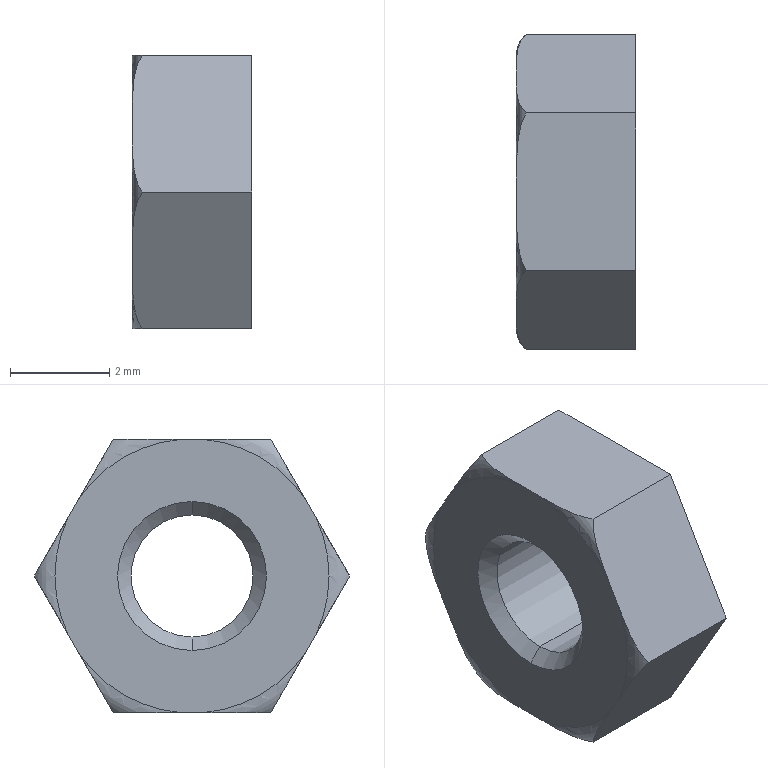Part | SolidWorks | features RefAxis 3, 3DProfileFeature 1, ICE 1, RevCut 1, Revolution 1 | 1 solid | 20 faces | box 2.4 x 6.351 x 5.5 mm | volume 50.814 mm3 | plane 8 | torus 6 | cone 4 | cylinder 2 | commonest cylinder face diameters 2.459 x2
STEP:
#1=CARTESIAN_POINT('',(0.9295,0.,-1.23));
#2=VERTEX_POINT('',#1);
#3=CARTESIAN_POINT('',(0.9295,0.,1.23));
#4=VERTEX_POINT('',#3);
#5=CARTESIAN_POINT('',(0.9295,0.,0.));
#6=DIRECTION('',(-1.,0.,0.));
#7=DIRECTION('',(0.,0.,1.));
#8=AXIS2_PLACEMENT_3D('',#5,#6,#7);
#9=CIRCLE('',#8,1.23);
#10=EDGE_CURVE('',#2,#4,#9,.T.);
#11=ORIENTED_EDGE('',*,*,#10,.T.);
#12=CARTESIAN_POINT('',(1.2,0.,1.5));
#13=VERTEX_POINT('',#12);
#14=CARTESIAN_POINT('',(1.2,0.,1.5));
#15=DIRECTION('',(0.7071,0.,0.7071));
#16=VECTOR('',#15,1000.);
#17=LINE('',#14,#16);
#18=EDGE_CURVE('',#4,#13,#17,.T.);
#19=ORIENTED_EDGE('',*,*,#18,.T.);
#20=CARTESIAN_POINT('',(1.2,0.,-1.5));
#21=VERTEX_POINT('',#20);
#22=CARTESIAN_POINT('',(1.2,0.,0.));
#23=DIRECTION('',(-1.,0.,0.));
#24=DIRECTION('',(0.,0.,1.));
#25=AXIS2_PLACEMENT_3D('',#22,#23,#24);
#26=CIRCLE('',#25,1.5);
#27=EDGE_CURVE('',#21,#13,#26,.T.);
#28=ORIENTED_EDGE('',*,*,#27,.F.);
#29=CARTESIAN_POINT('',(1.2,0.,-1.5));
#30=DIRECTION('',(0.7071,0.,-0.7071));
#31=VECTOR('',#30,1000.);
#32=LINE('',#29,#31);
#33=EDGE_CURVE('',#2,#21,#32,.T.);
#34=ORIENTED_EDGE('',*,*,#33,.F.);
#35=EDGE_LOOP('',(#11,#19,#28,#34));
#36=FACE_OUTER_BOUND('',#35,.T.);
#37=CARTESIAN_POINT('',(1.2,0.,0.));
#38=DIRECTION('',(1.,0.,0.));
#39=DIRECTION('',(0.,0.,-1.));
#40=AXIS2_PLACEMENT_3D('',#37,#38,#39);
#41=CONICAL_SURFACE('',#40,1.5,0.7854);
#42=ADVANCED_FACE('',(#36),#41,.F.);
#43=ORIENTED_EDGE('',*,*,#10,.F.);
#44=CARTESIAN_POINT('',(-0.9295,0.,-1.23));
#45=VERTEX_POINT('',#44);
#46=CARTESIAN_POINT('',(1.2,0.,-1.23));
#47=DIRECTION('',(-1.,0.,0.));
#48=VECTOR('',#47,1000.);
#49=LINE('',#46,#48);
#50=EDGE_CURVE('',#2,#45,#49,.T.);
#51=ORIENTED_EDGE('',*,*,#50,.T.);
#52=CARTESIAN_POINT('',(-0.9295,0.,1.23));
#53=VERTEX_POINT('',#52);
#54=CARTESIAN_POINT('',(-0.9295,0.,0.));
#55=DIRECTION('',(-1.,0.,0.));
#56=DIRECTION('',(0.,0.,1.));
#57=AXIS2_PLACEMENT_3D('',#54,#55,#56);
#58=CIRCLE('',#57,1.23);
#59=EDGE_CURVE('',#45,#53,#58,.T.);
#60=ORIENTED_EDGE('',*,*,#59,.T.);
#61=CARTESIAN_POINT('',(1.2,0.,1.23));
#62=DIRECTION('',(-1.,0.,0.));
#63=VECTOR('',#62,1000.);
#64=LINE('',#61,#63);
#65=EDGE_CURVE('',#4,#53,#64,.T.);
#66=ORIENTED_EDGE('',*,*,#65,.F.);
#67=EDGE_LOOP('',(#43,#51,#60,#66));
#68=FACE_OUTER_BOUND('',#67,.T.);
#69=CARTESIAN_POINT('',(1.2,0.,0.));
#70=DIRECTION('',(-1.,0.,0.));
#71=DIRECTION('',(0.,0.,1.));
#72=AXIS2_PLACEMENT_3D('',#69,#70,#71);
#73=CYLINDRICAL_SURFACE('',#72,1.23);
#74=ADVANCED_FACE('',(#68),#73,.F.);
#75=ORIENTED_EDGE('',*,*,#59,.F.);
#76=CARTESIAN_POINT('',(-1.2,0.,-1.5));
#77=VERTEX_POINT('',#76);
#78=CARTESIAN_POINT('',(-0.9295,0.,-1.23));
#79=DIRECTION('',(-0.7071,0.,-0.7071));
#80=VECTOR('',#79,1000.);
#81=LINE('',#78,#80);
#82=EDGE_CURVE('',#45,#77,#81,.T.);
#83=ORIENTED_EDGE('',*,*,#82,.T.);
#84=CARTESIAN_POINT('',(-1.2,0.,1.5));
#85=VERTEX_POINT('',#84);
#86=CARTESIAN_POINT('',(-1.2,0.,0.));
#87=DIRECTION('',(-1.,0.,0.));
#88=DIRECTION('',(0.,0.,1.));
#89=AXIS2_PLACEMENT_3D('',#86,#87,#88);
#90=CIRCLE('',#89,1.5);
#91=EDGE_CURVE('',#77,#85,#90,.T.);
#92=ORIENTED_EDGE('',*,*,#91,.T.);
#93=CARTESIAN_POINT('',(-0.9295,0.,1.23));
#94=DIRECTION('',(-0.7071,0.,0.7071));
#95=VECTOR('',#94,1000.);
#96=LINE('',#93,#95);
#97=EDGE_CURVE('',#53,#85,#96,.T.);
#98=ORIENTED_EDGE('',*,*,#97,.F.);
#99=EDGE_LOOP('',(#75,#83,#92,#98));
#100=FACE_OUTER_BOUND('',#99,.T.);
#101=CARTESIAN_POINT('',(-0.9295,0.,0.));
#102=DIRECTION('',(-1.,0.,0.));
#103=DIRECTION('',(0.,0.,1.));
#104=AXIS2_PLACEMENT_3D('',#101,#102,#103);
#105=CONICAL_SURFACE('',#104,1.23,0.7854);
#106=ADVANCED_FACE('',(#100),#105,.F.);
#107=CARTESIAN_POINT('',(-1.2,0.,0.));
#108=DIRECTION('',(-1.,0.,0.));
#109=DIRECTION('',(0.,0.,1.));
#110=AXIS2_PLACEMENT_3D('',#107,#108,#109);
#111=CIRCLE('',#110,1.5);
#112=EDGE_CURVE('',#85,#77,#111,.T.);
#113=ORIENTED_EDGE('',*,*,#112,.F.);
#114=ORIENTED_EDGE('',*,*,#91,.F.);
#115=EDGE_LOOP('',(#113,#114));
#116=FACE_BOUND('',#115,.T.);
#117=CARTESIAN_POINT('',(-1.2,2.499,1.172));
#118=VERTEX_POINT('',#117);
#119=CARTESIAN_POINT('',(-1.2,2.264,1.578));
#120=VERTEX_POINT('',#119);
#121=CARTESIAN_POINT('',(-1.2,3.175,0.));
#122=DIRECTION('',(0.,-0.5,0.866));
#123=VECTOR('',#122,1000.);
#124=LINE('',#121,#123);
#125=EDGE_CURVE('',#118,#120,#124,.T.);
#126=ORIENTED_EDGE('',*,*,#125,.F.);
#127=CARTESIAN_POINT('',(-1.2,2.499,-1.172));
#128=VERTEX_POINT('',#127);
#129=CARTESIAN_POINT('',(-1.2,0.,0.));
#130=DIRECTION('',(-1.,0.,0.));
#131=DIRECTION('',(0.,0.,1.));
#132=AXIS2_PLACEMENT_3D('',#129,#130,#131);
#133=CIRCLE('',#132,2.76);
#134=EDGE_CURVE('',#118,#128,#133,.T.);
#135=ORIENTED_EDGE('',*,*,#134,.T.);
#136=CARTESIAN_POINT('',(-1.2,2.264,-1.578));
#137=VERTEX_POINT('',#136);
#138=CARTESIAN_POINT('',(-1.2,1.588,-2.75));
#139=DIRECTION('',(0.,0.5,0.866));
#140=VECTOR('',#139,1000.);
#141=LINE('',#138,#140);
#142=EDGE_CURVE('',#137,#128,#141,.T.);
#143=ORIENTED_EDGE('',*,*,#142,.F.);
#144=CARTESIAN_POINT('',(-1.2,0.2347,-2.75));
#145=VERTEX_POINT('',#144);
#146=CARTESIAN_POINT('',(-1.2,0.,0.));
#147=DIRECTION('',(-1.,0.,0.));
#148=DIRECTION('',(0.,0.,1.));
#149=AXIS2_PLACEMENT_3D('',#146,#147,#148);
#150=CIRCLE('',#149,2.76);
#151=EDGE_CURVE('',#137,#145,#150,.T.);
#152=ORIENTED_EDGE('',*,*,#151,.T.);
#153=CARTESIAN_POINT('',(-1.2,-0.2347,-2.75));
#154=VERTEX_POINT('',#153);
#155=CARTESIAN_POINT('',(-1.2,-1.588,-2.75));
#156=DIRECTION('',(0.,1.,0.));
#157=VECTOR('',#156,1000.);
#158=LINE('',#155,#157);
#159=EDGE_CURVE('',#154,#145,#158,.T.);
#160=ORIENTED_EDGE('',*,*,#159,.F.);
#161=CARTESIAN_POINT('',(-1.2,-2.264,-1.578));
#162=VERTEX_POINT('',#161);
#163=CARTESIAN_POINT('',(-1.2,0.,0.));
#164=DIRECTION('',(-1.,0.,0.));
#165=DIRECTION('',(0.,0.,1.));
#166=AXIS2_PLACEMENT_3D('',#163,#164,#165);
#167=CIRCLE('',#166,2.76);
#168=EDGE_CURVE('',#154,#162,#167,.T.);
#169=ORIENTED_EDGE('',*,*,#168,.T.);
#170=CARTESIAN_POINT('',(-1.2,-2.499,-1.172));
#171=VERTEX_POINT('',#170);
#172=CARTESIAN_POINT('',(-1.2,-3.175,0.));
#173=DIRECTION('',(0.,0.5,-0.866));
#174=VECTOR('',#173,1000.);
#175=LINE('',#172,#174);
#176=EDGE_CURVE('',#171,#162,#175,.T.);
#177=ORIENTED_EDGE('',*,*,#176,.F.);
#178=CARTESIAN_POINT('',(-1.2,-2.499,1.172));
#179=VERTEX_POINT('',#178);
#180=CARTESIAN_POINT('',(-1.2,0.,0.));
#181=DIRECTION('',(-1.,0.,0.));
#182=DIRECTION('',(0.,0.,1.));
#183=AXIS2_PLACEMENT_3D('',#180,#181,#182);
#184=CIRCLE('',#183,2.76);
#185=EDGE_CURVE('',#171,#179,#184,.T.);
#186=ORIENTED_EDGE('',*,*,#185,.T.);
#187=CARTESIAN_POINT('',(-1.2,-2.264,1.578));
#188=VERTEX_POINT('',#187);
#189=CARTESIAN_POINT('',(-1.2,-1.588,2.75));
#190=DIRECTION('',(0.,-0.5,-0.866));
#191=VECTOR('',#190,1000.);
#192=LINE('',#189,#191);
#193=EDGE_CURVE('',#188,#179,#192,.T.);
#194=ORIENTED_EDGE('',*,*,#193,.F.);
#195=CARTESIAN_POINT('',(-1.2,-0.2347,2.75));
#196=VERTEX_POINT('',#195);
#197=CARTESIAN_POINT('',(-1.2,0.,0.));
#198=DIRECTION('',(-1.,0.,0.));
#199=DIRECTION('',(0.,0.,1.));
#200=AXIS2_PLACEMENT_3D('',#197,#198,#199);
#201=CIRCLE('',#200,2.76);
#202=EDGE_CURVE('',#188,#196,#201,.T.);
#203=ORIENTED_EDGE('',*,*,#202,.T.);
#204=CARTESIAN_POINT('',(-1.2,0.2347,2.75));
#205=VERTEX_POINT('',#204);
#206=CARTESIAN_POINT('',(-1.2,1.588,2.75));
#207=DIRECTION('',(0.,-1.,0.));
#208=VECTOR('',#207,1000.);
#209=LINE('',#206,#208);
#210=EDGE_CURVE('',#205,#196,#209,.T.);
#211=ORIENTED_EDGE('',*,*,#210,.F.);
#212=CARTESIAN_POINT('',(-1.2,0.,0.));
#213=DIRECTION('',(-1.,0.,0.));
#214=DIRECTION('',(0.,0.,1.));
#215=AXIS2_PLACEMENT_3D('',#212,#213,#214);
#216=CIRCLE('',#215,2.76);
#217=EDGE_CURVE('',#205,#120,#216,.T.);
#218=ORIENTED_EDGE('',*,*,#217,.T.);
#219=EDGE_LOOP('',(#126,#135,#143,#152,#160,#169,#177,#186,#194,#203,#211,#218));
#220=FACE_OUTER_BOUND('',#219,.T.);
#221=CARTESIAN_POINT('',(-1.2,0.,0.));
#222=DIRECTION('',(1.,0.,0.));
#223=DIRECTION('',(0.,0.,-1.));
#224=AXIS2_PLACEMENT_3D('',#221,#222,#223);
#225=PLANE('',#224);
#226=ADVANCED_FACE('',(#116,#220),#225,.F.);
#227=ORIENTED_EDGE('',*,*,#27,.T.);
#228=CARTESIAN_POINT('',(1.2,0.,0.));
#229=DIRECTION('',(-1.,0.,0.));
#230=DIRECTION('',(0.,0.,1.));
#231=AXIS2_PLACEMENT_3D('',#228,#229,#230);
#232=CIRCLE('',#231,1.5);
#233=EDGE_CURVE('',#13,#21,#232,.T.);
#234=ORIENTED_EDGE('',*,*,#233,.T.);
#235=EDGE_LOOP('',(#227,#234));
#236=FACE_BOUND('',#235,.T.);
#237=CARTESIAN_POINT('',(1.2,3.175,0.));
#238=VERTEX_POINT('',#237);
#239=CARTESIAN_POINT('',(1.2,1.588,2.75));
#240=VERTEX_POINT('',#239);
#241=CARTESIAN_POINT('',(1.2,3.175,0.));
#242=DIRECTION('',(0.,-0.5,0.866));
#243=VECTOR('',#242,1000.);
#244=LINE('',#241,#243);
#245=EDGE_CURVE('',#238,#240,#244,.T.);
#246=ORIENTED_EDGE('',*,*,#245,.T.);
#247=CARTESIAN_POINT('',(1.2,-1.588,2.75));
#248=VERTEX_POINT('',#247);
#249=CARTESIAN_POINT('',(1.2,1.588,2.75));
#250=DIRECTION('',(0.,-1.,0.));
#251=VECTOR('',#250,1000.);
#252=LINE('',#249,#251);
#253=EDGE_CURVE('',#240,#248,#252,.T.);
#254=ORIENTED_EDGE('',*,*,#253,.T.);
#255=CARTESIAN_POINT('',(1.2,-3.175,0.));
#256=VERTEX_POINT('',#255);
#257=CARTESIAN_POINT('',(1.2,-1.588,2.75));
#258=DIRECTION('',(0.,-0.5,-0.866));
#259=VECTOR('',#258,1000.);
#260=LINE('',#257,#259);
#261=EDGE_CURVE('',#248,#256,#260,.T.);
#262=ORIENTED_EDGE('',*,*,#261,.T.);
#263=CARTESIAN_POINT('',(1.2,-1.588,-2.75));
#264=VERTEX_POINT('',#263);
#265=CARTESIAN_POINT('',(1.2,-3.175,0.));
#266=DIRECTION('',(0.,0.5,-0.866));
#267=VECTOR('',#266,1000.);
#268=LINE('',#265,#267);
#269=EDGE_CURVE('',#256,#264,#268,.T.);
#270=ORIENTED_EDGE('',*,*,#269,.T.);
#271=CARTESIAN_POINT('',(1.2,1.588,-2.75));
#272=VERTEX_POINT('',#271);
#273=CARTESIAN_POINT('',(1.2,-1.588,-2.75));
#274=DIRECTION('',(0.,1.,0.));
#275=VECTOR('',#274,1000.);
#276=LINE('',#273,#275);
#277=EDGE_CURVE('',#264,#272,#276,.T.);
#278=ORIENTED_EDGE('',*,*,#277,.T.);
#279=CARTESIAN_POINT('',(1.2,1.588,-2.75));
#280=DIRECTION('',(0.,0.5,0.866));
#281=VECTOR('',#280,1000.);
#282=LINE('',#279,#281);
#283=EDGE_CURVE('',#272,#238,#282,.T.);
#284=ORIENTED_EDGE('',*,*,#283,.T.);
#285=EDGE_LOOP('',(#246,#254,#262,#270,#278,#284));
#286=FACE_OUTER_BOUND('',#285,.T.);
#287=CARTESIAN_POINT('',(1.2,3.3,0.));
#288=DIRECTION('',(-1.,0.,0.));
#289=DIRECTION('',(0.,0.,1.));
#290=AXIS2_PLACEMENT_3D('',#287,#288,#289);
#291=PLANE('',#290);
#292=ADVANCED_FACE('',(#236,#286),#291,.F.);
#293=CARTESIAN_POINT('',(-1.005,3.175,0.));
#294=VERTEX_POINT('',#293);
#295=CARTESIAN_POINT('',(-1.005,3.175,0.));
#296=CARTESIAN_POINT('',(-1.065,3.125,0.08691));
#297=CARTESIAN_POINT('',(-1.103,3.071,0.1816));
#298=CARTESIAN_POINT('',(-1.156,2.957,0.3777));
#299=CARTESIAN_POINT('',(-1.171,2.9,0.4765));
#300=CARTESIAN_POINT('',(-1.201,2.729,0.7735));
#301=CARTESIAN_POINT('',(-1.2,2.614,0.9727));
#302=CARTESIAN_POINT('',(-1.2,2.499,1.172));
#303=B_SPLINE_CURVE_WITH_KNOTS('',3,(#295,#296,#297,#298,#299,#300,#301,#302),.UNSPECIFIED.,.F.,.F.,(4,2,2,4),(0.000000265,0.0003463,0.0006923,0.001384),.UNSPECIFIED.);
#304=EDGE_CURVE('',#294,#118,#303,.T.);
#305=ORIENTED_EDGE('',*,*,#304,.F.);
#306=CARTESIAN_POINT('',(-1.2,2.499,-1.172));
#307=CARTESIAN_POINT('',(-1.2,2.614,-0.9724));
#308=CARTESIAN_POINT('',(-1.201,2.729,-0.773));
#309=CARTESIAN_POINT('',(-1.171,2.901,-0.4746));
#310=CARTESIAN_POINT('',(-1.156,2.959,-0.3755));
#311=CARTESIAN_POINT('',(-1.103,3.07,-0.1823));
#312=CARTESIAN_POINT('',(-1.065,3.126,-0.08628));
#313=CARTESIAN_POINT('',(-1.005,3.175,0.));
#314=B_SPLINE_CURVE_WITH_KNOTS('',3,(#306,#307,#308,#309,#310,#311,#312,#313),.UNSPECIFIED.,.F.,.F.,(4,2,2,4),(0.001855,0.002548,0.002895,0.003241),.UNSPECIFIED.);
#315=EDGE_CURVE('',#128,#294,#314,.T.);
#316=ORIENTED_EDGE('',*,*,#315,.F.);
#317=ORIENTED_EDGE('',*,*,#134,.F.);
#318=EDGE_LOOP('',(#305,#316,#317));
#319=FACE_OUTER_BOUND('',#318,.T.);
#320=CARTESIAN_POINT('',(-0.66,0.,0.));
#321=DIRECTION('',(-1.,0.,0.));
#322=DIRECTION('',(0.,0.,1.));
#323=AXIS2_PLACEMENT_3D('',#320,#321,#322);
#324=TOROIDAL_SURFACE('',#323,2.76,0.54);
#325=ADVANCED_FACE('',(#319),#324,.T.);
#326=CARTESIAN_POINT('',(-1.005,1.588,-2.75));
#327=VERTEX_POINT('',#326);
#328=CARTESIAN_POINT('',(-1.005,1.588,-2.75));
#329=CARTESIAN_POINT('',(-1.065,1.638,-2.663));
#330=CARTESIAN_POINT('',(-1.103,1.693,-2.568));
#331=CARTESIAN_POINT('',(-1.156,1.806,-2.372));
#332=CARTESIAN_POINT('',(-1.171,1.863,-2.274));
#333=CARTESIAN_POINT('',(-1.201,2.034,-1.976));
#334=CARTESIAN_POINT('',(-1.2,2.149,-1.777));
#335=CARTESIAN_POINT('',(-1.2,2.264,-1.578));
#336=B_SPLINE_CURVE_WITH_KNOTS('',3,(#328,#329,#330,#331,#332,#333,#334,#335),.UNSPECIFIED.,.F.,.F.,(4,2,2,4),(0.000000265,0.0003463,0.0006923,0.001384),.UNSPECIFIED.);
#337=EDGE_CURVE('',#327,#137,#336,.T.);
#338=ORIENTED_EDGE('',*,*,#337,.F.);
#339=CARTESIAN_POINT('',(-1.2,0.2347,-2.75));
#340=CARTESIAN_POINT('',(-1.2,0.4649,-2.75));
#341=CARTESIAN_POINT('',(-1.201,0.695,-2.75));
#342=CARTESIAN_POINT('',(-1.171,1.039,-2.75));
#343=CARTESIAN_POINT('',(-1.156,1.154,-2.75));
#344=CARTESIAN_POINT('',(-1.103,1.378,-2.75));
#345=CARTESIAN_POINT('',(-1.065,1.488,-2.75));
#346=CARTESIAN_POINT('',(-1.005,1.588,-2.75));
#347=B_SPLINE_CURVE_WITH_KNOTS('',3,(#339,#340,#341,#342,#343,#344,#345,#346),.UNSPECIFIED.,.F.,.F.,(4,2,2,4),(0.0002346,0.0009246,0.00127,0.001615),.UNSPECIFIED.);
#348=EDGE_CURVE('',#145,#327,#347,.T.);
#349=ORIENTED_EDGE('',*,*,#348,.F.);
#350=ORIENTED_EDGE('',*,*,#151,.F.);
#351=EDGE_LOOP('',(#338,#349,#350));
#352=FACE_OUTER_BOUND('',#351,.T.);
#353=CARTESIAN_POINT('',(-0.66,0.,0.));
#354=DIRECTION('',(-1.,0.,0.));
#355=DIRECTION('',(0.,0.,1.));
#356=AXIS2_PLACEMENT_3D('',#353,#354,#355);
#357=TOROIDAL_SURFACE('',#356,2.76,0.54);
#358=ADVANCED_FACE('',(#352),#357,.T.);
#359=CARTESIAN_POINT('',(-1.005,-1.588,-2.75));
#360=VERTEX_POINT('',#359);
#361=CARTESIAN_POINT('',(-1.005,-1.588,-2.75));
#362=CARTESIAN_POINT('',(-1.065,-1.488,-2.75));
#363=CARTESIAN_POINT('',(-1.103,-1.377,-2.75));
#364=CARTESIAN_POINT('',(-1.156,-1.153,-2.75));
#365=CARTESIAN_POINT('',(-1.171,-1.039,-2.75));
#366=CARTESIAN_POINT('',(-1.201,-0.6962,-2.75));
#367=CARTESIAN_POINT('',(-1.2,-0.4651,-2.75));
#368=CARTESIAN_POINT('',(-1.2,-0.2347,-2.75));
#369=B_SPLINE_CURVE_WITH_KNOTS('',3,(#361,#362,#363,#364,#365,#366,#367,#368),.UNSPECIFIED.,.F.,.F.,(4,2,2,4),(0.006601,0.006949,0.007298,0.007994),.UNSPECIFIED.);
#370=EDGE_CURVE('',#360,#154,#369,.T.);
#371=ORIENTED_EDGE('',*,*,#370,.F.);
#372=CARTESIAN_POINT('',(-1.2,-2.264,-1.578));
#373=CARTESIAN_POINT('',(-1.2,-2.149,-1.778));
#374=CARTESIAN_POINT('',(-1.201,-2.034,-1.977));
#375=CARTESIAN_POINT('',(-1.171,-1.862,-2.275));
#376=CARTESIAN_POINT('',(-1.156,-1.805,-2.374));
#377=CARTESIAN_POINT('',(-1.103,-1.693,-2.568));
#378=CARTESIAN_POINT('',(-1.065,-1.638,-2.664));
#379=CARTESIAN_POINT('',(-1.005,-1.588,-2.75));
#380=B_SPLINE_CURVE_WITH_KNOTS('',3,(#372,#373,#374,#375,#376,#377,#378,#379),.UNSPECIFIED.,.F.,.F.,(4,2,2,4),(0.001855,0.002548,0.002895,0.003241),.UNSPECIFIED.);
#381=EDGE_CURVE('',#162,#360,#380,.T.);
#382=ORIENTED_EDGE('',*,*,#381,.F.);
#383=ORIENTED_EDGE('',*,*,#168,.F.);
#384=EDGE_LOOP('',(#371,#382,#383));
#385=FACE_OUTER_BOUND('',#384,.T.);
#386=CARTESIAN_POINT('',(-0.66,0.,0.));
#387=DIRECTION('',(-1.,0.,0.));
#388=DIRECTION('',(0.,0.,1.));
#389=AXIS2_PLACEMENT_3D('',#386,#387,#388);
#390=TOROIDAL_SURFACE('',#389,2.76,0.54);
#391=ADVANCED_FACE('',(#385),#390,.T.);
#392=CARTESIAN_POINT('',(-1.005,-3.175,0.));
#393=VERTEX_POINT('',#392);
#394=CARTESIAN_POINT('',(-1.005,-3.175,0.));
#395=CARTESIAN_POINT('',(-1.065,-3.125,-0.08691));
#396=CARTESIAN_POINT('',(-1.103,-3.071,-0.1816));
#397=CARTESIAN_POINT('',(-1.156,-2.957,-0.3777));
#398=CARTESIAN_POINT('',(-1.171,-2.9,-0.4765));
#399=CARTESIAN_POINT('',(-1.201,-2.729,-0.7735));
#400=CARTESIAN_POINT('',(-1.2,-2.614,-0.9727));
#401=CARTESIAN_POINT('',(-1.2,-2.499,-1.172));
#402=B_SPLINE_CURVE_WITH_KNOTS('',3,(#394,#395,#396,#397,#398,#399,#400,#401),.UNSPECIFIED.,.F.,.F.,(4,2,2,4),(0.000000265,0.0003463,0.0006923,0.001384),.UNSPECIFIED.);
#403=EDGE_CURVE('',#393,#171,#402,.T.);
#404=ORIENTED_EDGE('',*,*,#403,.F.);
#405=CARTESIAN_POINT('',(-1.2,-2.499,1.172));
#406=CARTESIAN_POINT('',(-1.2,-2.614,0.9724));
#407=CARTESIAN_POINT('',(-1.201,-2.729,0.773));
#408=CARTESIAN_POINT('',(-1.171,-2.901,0.4746));
#409=CARTESIAN_POINT('',(-1.156,-2.959,0.3755));
#410=CARTESIAN_POINT('',(-1.103,-3.07,0.1823));
#411=CARTESIAN_POINT('',(-1.065,-3.126,0.08628));
#412=CARTESIAN_POINT('',(-1.005,-3.175,0.));
#413=B_SPLINE_CURVE_WITH_KNOTS('',3,(#405,#406,#407,#408,#409,#410,#411,#412),.UNSPECIFIED.,.F.,.F.,(4,2,2,4),(0.001855,0.002548,0.002895,0.003241),.UNSPECIFIED.);
#414=EDGE_CURVE('',#179,#393,#413,.T.);
#415=ORIENTED_EDGE('',*,*,#414,.F.);
#416=ORIENTED_EDGE('',*,*,#185,.F.);
#417=EDGE_LOOP('',(#404,#415,#416));
#418=FACE_OUTER_BOUND('',#417,.T.);
#419=CARTESIAN_POINT('',(-0.66,0.,0.));
#420=DIRECTION('',(-1.,0.,0.));
#421=DIRECTION('',(0.,0.,1.));
#422=AXIS2_PLACEMENT_3D('',#419,#420,#421);
#423=TOROIDAL_SURFACE('',#422,2.76,0.54);
#424=ADVANCED_FACE('',(#418),#423,.T.);
#425=CARTESIAN_POINT('',(-1.005,-1.588,2.75));
#426=VERTEX_POINT('',#425);
#427=CARTESIAN_POINT('',(-1.005,-1.588,2.75));
#428=CARTESIAN_POINT('',(-1.065,-1.638,2.663));
#429=CARTESIAN_POINT('',(-1.103,-1.693,2.568));
#430=CARTESIAN_POINT('',(-1.156,-1.806,2.372));
#431=CARTESIAN_POINT('',(-1.171,-1.863,2.274));
#432=CARTESIAN_POINT('',(-1.201,-2.034,1.976));
#433=CARTESIAN_POINT('',(-1.2,-2.149,1.777));
#434=CARTESIAN_POINT('',(-1.2,-2.264,1.578));
#435=B_SPLINE_CURVE_WITH_KNOTS('',3,(#427,#428,#429,#430,#431,#432,#433,#434),.UNSPECIFIED.,.F.,.F.,(4,2,2,4),(0.000000265,0.0003463,0.0006923,0.001384),.UNSPECIFIED.);
#436=EDGE_CURVE('',#426,#188,#435,.T.);
#437=ORIENTED_EDGE('',*,*,#436,.F.);
#438=CARTESIAN_POINT('',(-1.2,-0.2347,2.75));
#439=CARTESIAN_POINT('',(-1.2,-0.4649,2.75));
#440=CARTESIAN_POINT('',(-1.201,-0.695,2.75));
#441=CARTESIAN_POINT('',(-1.171,-1.039,2.75));
#442=CARTESIAN_POINT('',(-1.156,-1.154,2.75));
#443=CARTESIAN_POINT('',(-1.103,-1.378,2.75));
#444=CARTESIAN_POINT('',(-1.065,-1.488,2.75));
#445=CARTESIAN_POINT('',(-1.005,-1.588,2.75));
#446=B_SPLINE_CURVE_WITH_KNOTS('',3,(#438,#439,#440,#441,#442,#443,#444,#445),.UNSPECIFIED.,.F.,.F.,(4,2,2,4),(0.0002346,0.0009246,0.00127,0.001615),.UNSPECIFIED.);
#447=EDGE_CURVE('',#196,#426,#446,.T.);
#448=ORIENTED_EDGE('',*,*,#447,.F.);
#449=ORIENTED_EDGE('',*,*,#202,.F.);
#450=EDGE_LOOP('',(#437,#448,#449));
#451=FACE_OUTER_BOUND('',#450,.T.);
#452=CARTESIAN_POINT('',(-0.66,0.,0.));
#453=DIRECTION('',(-1.,0.,0.));
#454=DIRECTION('',(0.,0.,1.));
#455=AXIS2_PLACEMENT_3D('',#452,#453,#454);
#456=TOROIDAL_SURFACE('',#455,2.76,0.54);
#457=ADVANCED_FACE('',(#451),#456,.T.);
#458=CARTESIAN_POINT('',(-1.005,1.588,2.75));
#459=VERTEX_POINT('',#458);
#460=CARTESIAN_POINT('',(-1.2,2.264,1.578));
#461=CARTESIAN_POINT('',(-1.2,2.149,1.778));
#462=CARTESIAN_POINT('',(-1.201,2.034,1.977));
#463=CARTESIAN_POINT('',(-1.171,1.862,2.275));
#464=CARTESIAN_POINT('',(-1.156,1.805,2.374));
#465=CARTESIAN_POINT('',(-1.103,1.693,2.568));
#466=CARTESIAN_POINT('',(-1.065,1.638,2.664));
#467=CARTESIAN_POINT('',(-1.005,1.588,2.75));
#468=B_SPLINE_CURVE_WITH_KNOTS('',3,(#460,#461,#462,#463,#464,#465,#466,#467),.UNSPECIFIED.,.F.,.F.,(4,2,2,4),(0.001855,0.002548,0.002895,0.003241),.UNSPECIFIED.);
#469=EDGE_CURVE('',#120,#459,#468,.T.);
#470=ORIENTED_EDGE('',*,*,#469,.F.);
#471=ORIENTED_EDGE('',*,*,#217,.F.);
#472=CARTESIAN_POINT('',(-1.005,1.588,2.75));
#473=CARTESIAN_POINT('',(-1.065,1.488,2.75));
#474=CARTESIAN_POINT('',(-1.103,1.377,2.75));
#475=CARTESIAN_POINT('',(-1.156,1.153,2.75));
#476=CARTESIAN_POINT('',(-1.171,1.039,2.75));
#477=CARTESIAN_POINT('',(-1.201,0.6962,2.75));
#478=CARTESIAN_POINT('',(-1.2,0.4651,2.75));
#479=CARTESIAN_POINT('',(-1.2,0.2347,2.75));
#480=B_SPLINE_CURVE_WITH_KNOTS('',3,(#472,#473,#474,#475,#476,#477,#478,#479),.UNSPECIFIED.,.F.,.F.,(4,2,2,4),(0.006601,0.006949,0.007298,0.007994),.UNSPECIFIED.);
#481=EDGE_CURVE('',#459,#205,#480,.T.);
#482=ORIENTED_EDGE('',*,*,#481,.F.);
#483=EDGE_LOOP('',(#470,#471,#482));
#484=FACE_OUTER_BOUND('',#483,.T.);
#485=CARTESIAN_POINT('',(-0.66,0.,0.));
#486=DIRECTION('',(-1.,0.,0.));
#487=DIRECTION('',(0.,0.,1.));
#488=AXIS2_PLACEMENT_3D('',#485,#486,#487);
#489=TOROIDAL_SURFACE('',#488,2.76,0.54);
#490=ADVANCED_FACE('',(#484),#489,.T.);
#491=ORIENTED_EDGE('',*,*,#82,.F.);
#492=CARTESIAN_POINT('',(-0.9295,0.,0.));
#493=DIRECTION('',(-1.,0.,0.));
#494=DIRECTION('',(0.,0.,1.));
#495=AXIS2_PLACEMENT_3D('',#492,#493,#494);
#496=CIRCLE('',#495,1.23);
#497=EDGE_CURVE('',#53,#45,#496,.T.);
#498=ORIENTED_EDGE('',*,*,#497,.F.);
#499=ORIENTED_EDGE('',*,*,#97,.T.);
#500=ORIENTED_EDGE('',*,*,#112,.T.);
#501=EDGE_LOOP('',(#491,#498,#499,#500));
#502=FACE_OUTER_BOUND('',#501,.T.);
#503=CARTESIAN_POINT('',(-0.9295,0.,0.));
#504=DIRECTION('',(-1.,0.,0.));
#505=DIRECTION('',(0.,0.,1.));
#506=AXIS2_PLACEMENT_3D('',#503,#504,#505);
#507=CONICAL_SURFACE('',#506,1.23,0.7854);
#508=ADVANCED_FACE('',(#502),#507,.F.);
#509=ORIENTED_EDGE('',*,*,#50,.F.);
#510=CARTESIAN_POINT('',(0.9295,0.,0.));
#511=DIRECTION('',(-1.,0.,0.));
#512=DIRECTION('',(0.,0.,1.));
#513=AXIS2_PLACEMENT_3D('',#510,#511,#512);
#514=CIRCLE('',#513,1.23);
#515=EDGE_CURVE('',#4,#2,#514,.T.);
#516=ORIENTED_EDGE('',*,*,#515,.F.);
#517=ORIENTED_EDGE('',*,*,#65,.T.);
#518=ORIENTED_EDGE('',*,*,#497,.T.);
#519=EDGE_LOOP('',(#509,#516,#517,#518));
#520=FACE_OUTER_BOUND('',#519,.T.);
#521=CARTESIAN_POINT('',(1.2,0.,0.));
#522=DIRECTION('',(-1.,0.,0.));
#523=DIRECTION('',(0.,0.,1.));
#524=AXIS2_PLACEMENT_3D('',#521,#522,#523);
#525=CYLINDRICAL_SURFACE('',#524,1.23);
#526=ADVANCED_FACE('',(#520),#525,.F.);
#527=ORIENTED_EDGE('',*,*,#18,.F.);
#528=ORIENTED_EDGE('',*,*,#515,.T.);
#529=ORIENTED_EDGE('',*,*,#33,.T.);
#530=ORIENTED_EDGE('',*,*,#233,.F.);
#531=EDGE_LOOP('',(#527,#528,#529,#530));
#532=FACE_OUTER_BOUND('',#531,.T.);
#533=CARTESIAN_POINT('',(1.2,0.,0.));
#534=DIRECTION('',(1.,0.,0.));
#535=DIRECTION('',(0.,0.,-1.));
#536=AXIS2_PLACEMENT_3D('',#533,#534,#535);
#537=CONICAL_SURFACE('',#536,1.5,0.7854);
#538=ADVANCED_FACE('',(#532),#537,.F.);
#539=ORIENTED_EDGE('',*,*,#304,.T.);
#540=ORIENTED_EDGE('',*,*,#125,.T.);
#541=ORIENTED_EDGE('',*,*,#469,.T.);
#542=CARTESIAN_POINT('',(-1.2,1.588,2.75));
#543=DIRECTION('',(1.,0.,0.));
#544=VECTOR('',#543,1000.);
#545=LINE('',#542,#544);
#546=EDGE_CURVE('',#459,#240,#545,.T.);
#547=ORIENTED_EDGE('',*,*,#546,.T.);
#548=ORIENTED_EDGE('',*,*,#245,.F.);
#549=CARTESIAN_POINT('',(-1.2,3.175,0.));
#550=DIRECTION('',(1.,0.,0.));
#551=VECTOR('',#550,1000.);
#552=LINE('',#549,#551);
#553=EDGE_CURVE('',#294,#238,#552,.T.);
#554=ORIENTED_EDGE('',*,*,#553,.F.);
#555=EDGE_LOOP('',(#539,#540,#541,#547,#548,#554));
#556=FACE_OUTER_BOUND('',#555,.T.);
#557=CARTESIAN_POINT('',(-1.2,3.175,0.));
#558=DIRECTION('',(0.,0.866,0.5));
#559=DIRECTION('',(0.,-0.5,0.866));
#560=AXIS2_PLACEMENT_3D('',#557,#558,#559);
#561=PLANE('',#560);
#562=ADVANCED_FACE('',(#556),#561,.T.);
#563=ORIENTED_EDGE('',*,*,#337,.T.);
#564=ORIENTED_EDGE('',*,*,#142,.T.);
#565=ORIENTED_EDGE('',*,*,#315,.T.);
#566=ORIENTED_EDGE('',*,*,#553,.T.);
#567=ORIENTED_EDGE('',*,*,#283,.F.);
#568=CARTESIAN_POINT('',(-1.2,1.588,-2.75));
#569=DIRECTION('',(1.,0.,0.));
#570=VECTOR('',#569,1000.);
#571=LINE('',#568,#570);
#572=EDGE_CURVE('',#327,#272,#571,.T.);
#573=ORIENTED_EDGE('',*,*,#572,.F.);
#574=EDGE_LOOP('',(#563,#564,#565,#566,#567,#573));
#575=FACE_OUTER_BOUND('',#574,.T.);
#576=CARTESIAN_POINT('',(-1.2,1.588,-2.75));
#577=DIRECTION('',(0.,0.866,-0.5));
#578=DIRECTION('',(0.,0.5,0.866));
#579=AXIS2_PLACEMENT_3D('',#576,#577,#578);
#580=PLANE('',#579);
#581=ADVANCED_FACE('',(#575),#580,.T.);
#582=ORIENTED_EDGE('',*,*,#348,.T.);
#583=ORIENTED_EDGE('',*,*,#572,.T.);
#584=ORIENTED_EDGE('',*,*,#277,.F.);
#585=CARTESIAN_POINT('',(-1.2,-1.588,-2.75));
#586=DIRECTION('',(1.,0.,0.));
#587=VECTOR('',#586,1000.);
#588=LINE('',#585,#587);
#589=EDGE_CURVE('',#360,#264,#588,.T.);
#590=ORIENTED_EDGE('',*,*,#589,.F.);
#591=ORIENTED_EDGE('',*,*,#370,.T.);
#592=ORIENTED_EDGE('',*,*,#159,.T.);
#593=EDGE_LOOP('',(#582,#583,#584,#590,#591,#592));
#594=FACE_OUTER_BOUND('',#593,.T.);
#595=CARTESIAN_POINT('',(-1.2,-1.588,-2.75));
#596=DIRECTION('',(0.,0.,-1.));
#597=DIRECTION('',(-1.,0.,0.));
#598=AXIS2_PLACEMENT_3D('',#595,#596,#597);
#599=PLANE('',#598);
#600=ADVANCED_FACE('',(#594),#599,.T.);
#601=ORIENTED_EDGE('',*,*,#403,.T.);
#602=ORIENTED_EDGE('',*,*,#176,.T.);
#603=ORIENTED_EDGE('',*,*,#381,.T.);
#604=ORIENTED_EDGE('',*,*,#589,.T.);
#605=ORIENTED_EDGE('',*,*,#269,.F.);
#606=CARTESIAN_POINT('',(-1.2,-3.175,0.));
#607=DIRECTION('',(1.,0.,0.));
#608=VECTOR('',#607,1000.);
#609=LINE('',#606,#608);
#610=EDGE_CURVE('',#393,#256,#609,.T.);
#611=ORIENTED_EDGE('',*,*,#610,.F.);
#612=EDGE_LOOP('',(#601,#602,#603,#604,#605,#611));
#613=FACE_OUTER_BOUND('',#612,.T.);
#614=CARTESIAN_POINT('',(-1.2,-3.175,0.));
#615=DIRECTION('',(0.,-0.866,-0.5));
#616=DIRECTION('',(0.,0.5,-0.866));
#617=AXIS2_PLACEMENT_3D('',#614,#615,#616);
#618=PLANE('',#617);
#619=ADVANCED_FACE('',(#613),#618,.T.);
#620=ORIENTED_EDGE('',*,*,#436,.T.);
#621=ORIENTED_EDGE('',*,*,#193,.T.);
#622=ORIENTED_EDGE('',*,*,#414,.T.);
#623=ORIENTED_EDGE('',*,*,#610,.T.);
#624=ORIENTED_EDGE('',*,*,#261,.F.);
#625=CARTESIAN_POINT('',(-1.2,-1.588,2.75));
#626=DIRECTION('',(1.,0.,0.));
#627=VECTOR('',#626,1000.);
#628=LINE('',#625,#627);
#629=EDGE_CURVE('',#426,#248,#628,.T.);
#630=ORIENTED_EDGE('',*,*,#629,.F.);
#631=EDGE_LOOP('',(#620,#621,#622,#623,#624,#630));
#632=FACE_OUTER_BOUND('',#631,.T.);
#633=CARTESIAN_POINT('',(-1.2,-1.588,2.75));
#634=DIRECTION('',(0.,-0.866,0.5));
#635=DIRECTION('',(0.,-0.5,-0.866));
#636=AXIS2_PLACEMENT_3D('',#633,#634,#635);
#637=PLANE('',#636);
#638=ADVANCED_FACE('',(#632),#637,.T.);
#639=ORIENTED_EDGE('',*,*,#447,.T.);
#640=ORIENTED_EDGE('',*,*,#629,.T.);
#641=ORIENTED_EDGE('',*,*,#253,.F.);
#642=ORIENTED_EDGE('',*,*,#546,.F.);
#643=ORIENTED_EDGE('',*,*,#481,.T.);
#644=ORIENTED_EDGE('',*,*,#210,.T.);
#645=EDGE_LOOP('',(#639,#640,#641,#642,#643,#644));
#646=FACE_OUTER_BOUND('',#645,.T.);
#647=CARTESIAN_POINT('',(-1.2,1.588,2.75));
#648=DIRECTION('',(0.,0.,1.));
#649=DIRECTION('',(1.,0.,0.));
#650=AXIS2_PLACEMENT_3D('',#647,#648,#649);
#651=PLANE('',#650);
#652=ADVANCED_FACE('',(#646),#651,.T.);
#653=CLOSED_SHELL('',(#42,#74,#106,#226,#292,#325,#358,#391,#424,#457,#490,#508,#526,#538,#562,#581,#600,#619,#638,#652));
#654=MANIFOLD_SOLID_BREP('',#653);
#655=CARTESIAN_POINT('',(0.,0.,0.));
#656=DIRECTION('',(0.,0.,1.));
#657=DIRECTION('',(1.,0.,0.));
#658=AXIS2_PLACEMENT_3D('',#655,#656,#657);
#659=(LENGTH_UNIT()NAMED_UNIT(*)SI_UNIT(.MILLI.,.METRE.));
#660=UNCERTAINTY_MEASURE_WITH_UNIT(LENGTH_MEASURE(0.00001),#659,'','');
#661=(NAMED_UNIT(*)PLANE_ANGLE_UNIT()SI_UNIT($,.RADIAN.));
#662=(NAMED_UNIT(*)SI_UNIT($,.STERADIAN.)SOLID_ANGLE_UNIT());
#663=(GEOMETRIC_REPRESENTATION_CONTEXT(3)GLOBAL_UNCERTAINTY_ASSIGNED_CONTEXT((#660))GLOBAL_UNIT_ASSIGNED_CONTEXT((#659,#661,#662))REPRESENTATION_CONTEXT('',''));
#664=ADVANCED_BREP_SHAPE_REPRESENTATION('',(#654,#658),#663);